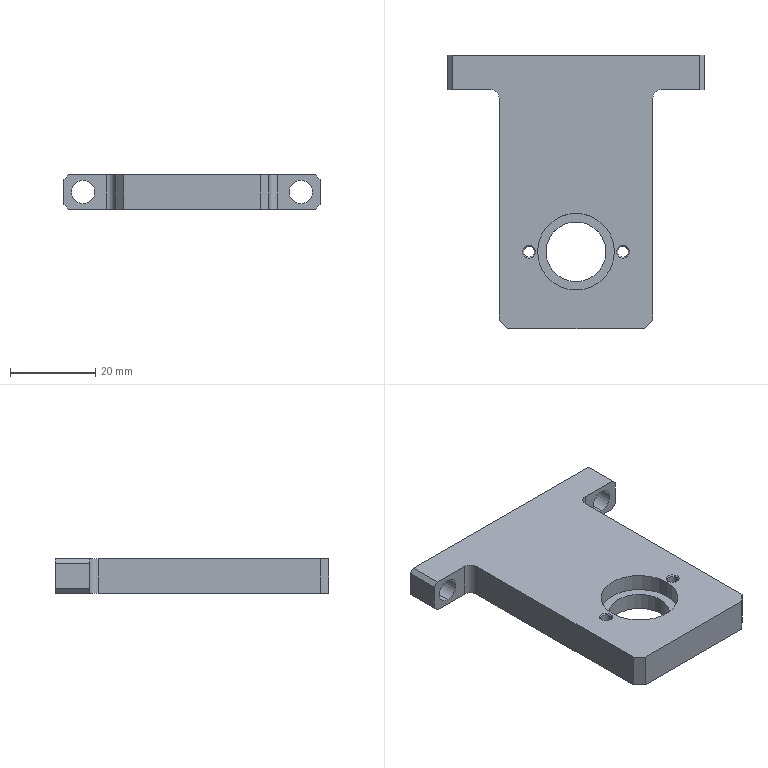Part | STEP file | FBDS-CS-017 | 1 solid | 35 faces | box 60 x 64 x 8 mm | volume 17841 mm3 | plane 17 | cylinder 14 | cone 4 | commonest cylinder face diameters 2.5 x4 5.5 x4 4 x2 14 x2 18 x2
STEP:
#1=CARTESIAN_POINT('',(-12.25,-14.,7.725));
#2=VERTEX_POINT('',#1);
#3=CARTESIAN_POINT('',(-9.75,-14.,7.725));
#4=VERTEX_POINT('',#3);
#5=CARTESIAN_POINT('',(-11.,-14.,7.725));
#6=DIRECTION('',(0.,0.,1.));
#7=DIRECTION('',(1.,0.,0.));
#8=AXIS2_PLACEMENT_3D('',#5,#6,#7);
#9=CIRCLE('',#8,1.25);
#10=EDGE_CURVE('',#2,#4,#9,.T.);
#11=ORIENTED_EDGE('',*,*,#10,.F.);
#12=CARTESIAN_POINT('',(-12.525,-14.,8.));
#13=VERTEX_POINT('',#12);
#14=CARTESIAN_POINT('',(-12.525,-14.,8.));
#15=DIRECTION('',(-0.7071,0.,0.7071));
#16=VECTOR('',#15,1000.);
#17=LINE('',#14,#16);
#18=EDGE_CURVE('',#2,#13,#17,.T.);
#19=ORIENTED_EDGE('',*,*,#18,.T.);
#20=CARTESIAN_POINT('',(-9.475,-14.,8.));
#21=VERTEX_POINT('',#20);
#22=CARTESIAN_POINT('',(-11.,-14.,8.));
#23=DIRECTION('',(0.,0.,1.));
#24=DIRECTION('',(1.,0.,0.));
#25=AXIS2_PLACEMENT_3D('',#22,#23,#24);
#26=CIRCLE('',#25,1.525);
#27=EDGE_CURVE('',#13,#21,#26,.T.);
#28=ORIENTED_EDGE('',*,*,#27,.T.);
#29=CARTESIAN_POINT('',(-9.475,-14.,8.));
#30=DIRECTION('',(0.7071,0.,0.7071));
#31=VECTOR('',#30,1000.);
#32=LINE('',#29,#31);
#33=EDGE_CURVE('',#4,#21,#32,.T.);
#34=ORIENTED_EDGE('',*,*,#33,.F.);
#35=EDGE_LOOP('',(#11,#19,#28,#34));
#36=FACE_OUTER_BOUND('',#35,.T.);
#37=CARTESIAN_POINT('',(-11.,-14.,8.));
#38=DIRECTION('',(0.,0.,1.));
#39=DIRECTION('',(1.,0.,0.));
#40=AXIS2_PLACEMENT_3D('',#37,#38,#39);
#41=CONICAL_SURFACE('',#40,1.525,0.7854);
#42=ADVANCED_FACE('',(#36),#41,.F.);
#43=CARTESIAN_POINT('',(-12.25,-14.,0.));
#44=VERTEX_POINT('',#43);
#45=CARTESIAN_POINT('',(-9.75,-14.,0.));
#46=VERTEX_POINT('',#45);
#47=CARTESIAN_POINT('',(-11.,-14.,0.));
#48=DIRECTION('',(0.,0.,1.));
#49=DIRECTION('',(1.,0.,0.));
#50=AXIS2_PLACEMENT_3D('',#47,#48,#49);
#51=CIRCLE('',#50,1.25);
#52=EDGE_CURVE('',#44,#46,#51,.T.);
#53=ORIENTED_EDGE('',*,*,#52,.F.);
#54=CARTESIAN_POINT('',(-12.25,-14.,8.));
#55=DIRECTION('',(0.,0.,1.));
#56=VECTOR('',#55,1000.);
#57=LINE('',#54,#56);
#58=EDGE_CURVE('',#44,#2,#57,.T.);
#59=ORIENTED_EDGE('',*,*,#58,.T.);
#60=ORIENTED_EDGE('',*,*,#10,.T.);
#61=CARTESIAN_POINT('',(-9.75,-14.,8.));
#62=DIRECTION('',(0.,0.,1.));
#63=VECTOR('',#62,1000.);
#64=LINE('',#61,#63);
#65=EDGE_CURVE('',#46,#4,#64,.T.);
#66=ORIENTED_EDGE('',*,*,#65,.F.);
#67=EDGE_LOOP('',(#53,#59,#60,#66));
#68=FACE_OUTER_BOUND('',#67,.T.);
#69=CARTESIAN_POINT('',(-11.,-14.,8.));
#70=DIRECTION('',(0.,0.,1.));
#71=DIRECTION('',(1.,0.,0.));
#72=AXIS2_PLACEMENT_3D('',#69,#70,#71);
#73=CYLINDRICAL_SURFACE('',#72,1.25);
#74=ADVANCED_FACE('',(#68),#73,.F.);
#75=CARTESIAN_POINT('',(9.75,-14.,7.725));
#76=VERTEX_POINT('',#75);
#77=CARTESIAN_POINT('',(12.25,-14.,7.725));
#78=VERTEX_POINT('',#77);
#79=CARTESIAN_POINT('',(11.,-14.,7.725));
#80=DIRECTION('',(0.,0.,1.));
#81=DIRECTION('',(1.,0.,0.));
#82=AXIS2_PLACEMENT_3D('',#79,#80,#81);
#83=CIRCLE('',#82,1.25);
#84=EDGE_CURVE('',#76,#78,#83,.T.);
#85=ORIENTED_EDGE('',*,*,#84,.F.);
#86=CARTESIAN_POINT('',(9.475,-14.,8.));
#87=VERTEX_POINT('',#86);
#88=CARTESIAN_POINT('',(9.475,-14.,8.));
#89=DIRECTION('',(-0.7071,0.,0.7071));
#90=VECTOR('',#89,1000.);
#91=LINE('',#88,#90);
#92=EDGE_CURVE('',#76,#87,#91,.T.);
#93=ORIENTED_EDGE('',*,*,#92,.T.);
#94=CARTESIAN_POINT('',(12.525,-14.,8.));
#95=VERTEX_POINT('',#94);
#96=CARTESIAN_POINT('',(11.,-14.,8.));
#97=DIRECTION('',(0.,0.,1.));
#98=DIRECTION('',(1.,0.,0.));
#99=AXIS2_PLACEMENT_3D('',#96,#97,#98);
#100=CIRCLE('',#99,1.525);
#101=EDGE_CURVE('',#87,#95,#100,.T.);
#102=ORIENTED_EDGE('',*,*,#101,.T.);
#103=CARTESIAN_POINT('',(12.525,-14.,8.));
#104=DIRECTION('',(0.7071,0.,0.7071));
#105=VECTOR('',#104,1000.);
#106=LINE('',#103,#105);
#107=EDGE_CURVE('',#78,#95,#106,.T.);
#108=ORIENTED_EDGE('',*,*,#107,.F.);
#109=EDGE_LOOP('',(#85,#93,#102,#108));
#110=FACE_OUTER_BOUND('',#109,.T.);
#111=CARTESIAN_POINT('',(11.,-14.,8.));
#112=DIRECTION('',(0.,0.,1.));
#113=DIRECTION('',(1.,0.,0.));
#114=AXIS2_PLACEMENT_3D('',#111,#112,#113);
#115=CONICAL_SURFACE('',#114,1.525,0.7854);
#116=ADVANCED_FACE('',(#110),#115,.F.);
#117=CARTESIAN_POINT('',(9.75,-14.,0.));
#118=VERTEX_POINT('',#117);
#119=CARTESIAN_POINT('',(12.25,-14.,0.));
#120=VERTEX_POINT('',#119);
#121=CARTESIAN_POINT('',(11.,-14.,0.));
#122=DIRECTION('',(0.,0.,1.));
#123=DIRECTION('',(1.,0.,0.));
#124=AXIS2_PLACEMENT_3D('',#121,#122,#123);
#125=CIRCLE('',#124,1.25);
#126=EDGE_CURVE('',#118,#120,#125,.T.);
#127=ORIENTED_EDGE('',*,*,#126,.F.);
#128=CARTESIAN_POINT('',(9.75,-14.,8.));
#129=DIRECTION('',(0.,0.,1.));
#130=VECTOR('',#129,1000.);
#131=LINE('',#128,#130);
#132=EDGE_CURVE('',#118,#76,#131,.T.);
#133=ORIENTED_EDGE('',*,*,#132,.T.);
#134=ORIENTED_EDGE('',*,*,#84,.T.);
#135=CARTESIAN_POINT('',(12.25,-14.,8.));
#136=DIRECTION('',(0.,0.,1.));
#137=VECTOR('',#136,1000.);
#138=LINE('',#135,#137);
#139=EDGE_CURVE('',#120,#78,#138,.T.);
#140=ORIENTED_EDGE('',*,*,#139,.F.);
#141=EDGE_LOOP('',(#127,#133,#134,#140));
#142=FACE_OUTER_BOUND('',#141,.T.);
#143=CARTESIAN_POINT('',(11.,-14.,8.));
#144=DIRECTION('',(0.,0.,1.));
#145=DIRECTION('',(1.,0.,0.));
#146=AXIS2_PLACEMENT_3D('',#143,#144,#145);
#147=CYLINDRICAL_SURFACE('',#146,1.25);
#148=ADVANCED_FACE('',(#142),#147,.F.);
#149=CARTESIAN_POINT('',(-25.5,32.,6.75));
#150=VERTEX_POINT('',#149);
#151=CARTESIAN_POINT('',(-25.5,32.,1.25));
#152=VERTEX_POINT('',#151);
#153=CARTESIAN_POINT('',(-25.5,32.,4.));
#154=DIRECTION('',(0.,-1.,0.));
#155=DIRECTION('',(0.,0.,-1.));
#156=AXIS2_PLACEMENT_3D('',#153,#154,#155);
#157=CIRCLE('',#156,2.75);
#158=EDGE_CURVE('',#150,#152,#157,.T.);
#159=ORIENTED_EDGE('',*,*,#158,.F.);
#160=CARTESIAN_POINT('',(-25.5,24.,6.75));
#161=VERTEX_POINT('',#160);
#162=CARTESIAN_POINT('',(-25.5,24.,6.75));
#163=DIRECTION('',(0.,-1.,0.));
#164=VECTOR('',#163,1000.);
#165=LINE('',#162,#164);
#166=EDGE_CURVE('',#150,#161,#165,.T.);
#167=ORIENTED_EDGE('',*,*,#166,.T.);
#168=CARTESIAN_POINT('',(-25.5,24.,1.25));
#169=VERTEX_POINT('',#168);
#170=CARTESIAN_POINT('',(-25.5,24.,4.));
#171=DIRECTION('',(0.,-1.,0.));
#172=DIRECTION('',(0.,0.,-1.));
#173=AXIS2_PLACEMENT_3D('',#170,#171,#172);
#174=CIRCLE('',#173,2.75);
#175=EDGE_CURVE('',#161,#169,#174,.T.);
#176=ORIENTED_EDGE('',*,*,#175,.T.);
#177=CARTESIAN_POINT('',(-25.5,24.,1.25));
#178=DIRECTION('',(0.,-1.,0.));
#179=VECTOR('',#178,1000.);
#180=LINE('',#177,#179);
#181=EDGE_CURVE('',#152,#169,#180,.T.);
#182=ORIENTED_EDGE('',*,*,#181,.F.);
#183=EDGE_LOOP('',(#159,#167,#176,#182));
#184=FACE_OUTER_BOUND('',#183,.T.);
#185=CARTESIAN_POINT('',(-25.5,24.,4.));
#186=DIRECTION('',(0.,-1.,0.));
#187=DIRECTION('',(0.,0.,-1.));
#188=AXIS2_PLACEMENT_3D('',#185,#186,#187);
#189=CYLINDRICAL_SURFACE('',#188,2.75);
#190=ADVANCED_FACE('',(#184),#189,.F.);
#191=CARTESIAN_POINT('',(25.5,32.,6.75));
#192=VERTEX_POINT('',#191);
#193=CARTESIAN_POINT('',(25.5,32.,1.25));
#194=VERTEX_POINT('',#193);
#195=CARTESIAN_POINT('',(25.5,32.,4.));
#196=DIRECTION('',(0.,-1.,0.));
#197=DIRECTION('',(0.,0.,-1.));
#198=AXIS2_PLACEMENT_3D('',#195,#196,#197);
#199=CIRCLE('',#198,2.75);
#200=EDGE_CURVE('',#192,#194,#199,.T.);
#201=ORIENTED_EDGE('',*,*,#200,.F.);
#202=CARTESIAN_POINT('',(25.5,24.,6.75));
#203=VERTEX_POINT('',#202);
#204=CARTESIAN_POINT('',(25.5,24.,6.75));
#205=DIRECTION('',(0.,-1.,0.));
#206=VECTOR('',#205,1000.);
#207=LINE('',#204,#206);
#208=EDGE_CURVE('',#192,#203,#207,.T.);
#209=ORIENTED_EDGE('',*,*,#208,.T.);
#210=CARTESIAN_POINT('',(25.5,24.,1.25));
#211=VERTEX_POINT('',#210);
#212=CARTESIAN_POINT('',(25.5,24.,4.));
#213=DIRECTION('',(0.,-1.,0.));
#214=DIRECTION('',(0.,0.,-1.));
#215=AXIS2_PLACEMENT_3D('',#212,#213,#214);
#216=CIRCLE('',#215,2.75);
#217=EDGE_CURVE('',#203,#211,#216,.T.);
#218=ORIENTED_EDGE('',*,*,#217,.T.);
#219=CARTESIAN_POINT('',(25.5,24.,1.25));
#220=DIRECTION('',(0.,-1.,0.));
#221=VECTOR('',#220,1000.);
#222=LINE('',#219,#221);
#223=EDGE_CURVE('',#194,#211,#222,.T.);
#224=ORIENTED_EDGE('',*,*,#223,.F.);
#225=EDGE_LOOP('',(#201,#209,#218,#224));
#226=FACE_OUTER_BOUND('',#225,.T.);
#227=CARTESIAN_POINT('',(25.5,24.,4.));
#228=DIRECTION('',(0.,-1.,0.));
#229=DIRECTION('',(0.,0.,-1.));
#230=AXIS2_PLACEMENT_3D('',#227,#228,#229);
#231=CYLINDRICAL_SURFACE('',#230,2.75);
#232=ADVANCED_FACE('',(#226),#231,.F.);
#233=CARTESIAN_POINT('',(7.,-14.,4.));
#234=VERTEX_POINT('',#233);
#235=CARTESIAN_POINT('',(-7.,-14.,4.));
#236=VERTEX_POINT('',#235);
#237=CARTESIAN_POINT('',(0.,-14.,4.));
#238=DIRECTION('',(0.,0.,-1.));
#239=DIRECTION('',(-1.,0.,0.));
#240=AXIS2_PLACEMENT_3D('',#237,#238,#239);
#241=CIRCLE('',#240,7.);
#242=EDGE_CURVE('',#234,#236,#241,.T.);
#243=ORIENTED_EDGE('',*,*,#242,.F.);
#244=CARTESIAN_POINT('',(7.,-14.,0.));
#245=VERTEX_POINT('',#244);
#246=CARTESIAN_POINT('',(7.,-14.,4.));
#247=DIRECTION('',(0.,0.,-1.));
#248=VECTOR('',#247,1000.);
#249=LINE('',#246,#248);
#250=EDGE_CURVE('',#234,#245,#249,.T.);
#251=ORIENTED_EDGE('',*,*,#250,.T.);
#252=CARTESIAN_POINT('',(-7.,-14.,0.));
#253=VERTEX_POINT('',#252);
#254=CARTESIAN_POINT('',(0.,-14.,0.));
#255=DIRECTION('',(0.,0.,-1.));
#256=DIRECTION('',(-1.,0.,0.));
#257=AXIS2_PLACEMENT_3D('',#254,#255,#256);
#258=CIRCLE('',#257,7.);
#259=EDGE_CURVE('',#245,#253,#258,.T.);
#260=ORIENTED_EDGE('',*,*,#259,.T.);
#261=CARTESIAN_POINT('',(-7.,-14.,4.));
#262=DIRECTION('',(0.,0.,-1.));
#263=VECTOR('',#262,1000.);
#264=LINE('',#261,#263);
#265=EDGE_CURVE('',#236,#253,#264,.T.);
#266=ORIENTED_EDGE('',*,*,#265,.F.);
#267=EDGE_LOOP('',(#243,#251,#260,#266));
#268=FACE_OUTER_BOUND('',#267,.T.);
#269=CARTESIAN_POINT('',(0.,-14.,4.));
#270=DIRECTION('',(0.,0.,-1.));
#271=DIRECTION('',(-1.,0.,0.));
#272=AXIS2_PLACEMENT_3D('',#269,#270,#271);
#273=CYLINDRICAL_SURFACE('',#272,7.);
#274=ADVANCED_FACE('',(#268),#273,.F.);
#275=CARTESIAN_POINT('',(-9.,-14.,4.));
#276=VERTEX_POINT('',#275);
#277=CARTESIAN_POINT('',(9.,-14.,4.));
#278=VERTEX_POINT('',#277);
#279=CARTESIAN_POINT('',(0.,-14.,4.));
#280=DIRECTION('',(0.,0.,1.));
#281=DIRECTION('',(-1.,0.,0.));
#282=AXIS2_PLACEMENT_3D('',#279,#280,#281);
#283=CIRCLE('',#282,9.);
#284=EDGE_CURVE('',#276,#278,#283,.T.);
#285=ORIENTED_EDGE('',*,*,#284,.F.);
#286=CARTESIAN_POINT('',(-9.,-14.,8.));
#287=VERTEX_POINT('',#286);
#288=CARTESIAN_POINT('',(-9.,-14.,-2.));
#289=DIRECTION('',(0.,0.,1.));
#290=VECTOR('',#289,1000.);
#291=LINE('',#288,#290);
#292=EDGE_CURVE('',#276,#287,#291,.T.);
#293=ORIENTED_EDGE('',*,*,#292,.T.);
#294=CARTESIAN_POINT('',(9.,-14.,8.));
#295=VERTEX_POINT('',#294);
#296=CARTESIAN_POINT('',(0.,-14.,8.));
#297=DIRECTION('',(0.,0.,1.));
#298=DIRECTION('',(1.,0.,0.));
#299=AXIS2_PLACEMENT_3D('',#296,#297,#298);
#300=CIRCLE('',#299,9.);
#301=EDGE_CURVE('',#287,#295,#300,.T.);
#302=ORIENTED_EDGE('',*,*,#301,.T.);
#303=CARTESIAN_POINT('',(9.,-14.,-2.));
#304=DIRECTION('',(0.,0.,1.));
#305=VECTOR('',#304,1000.);
#306=LINE('',#303,#305);
#307=EDGE_CURVE('',#278,#295,#306,.T.);
#308=ORIENTED_EDGE('',*,*,#307,.F.);
#309=EDGE_LOOP('',(#285,#293,#302,#308));
#310=FACE_OUTER_BOUND('',#309,.T.);
#311=CARTESIAN_POINT('',(0.,-14.,-2.));
#312=DIRECTION('',(0.,0.,1.));
#313=DIRECTION('',(1.,0.,0.));
#314=AXIS2_PLACEMENT_3D('',#311,#312,#313);
#315=CYLINDRICAL_SURFACE('',#314,9.);
#316=ADVANCED_FACE('',(#310),#315,.F.);
#317=ORIENTED_EDGE('',*,*,#292,.F.);
#318=CARTESIAN_POINT('',(0.,-14.,4.));
#319=DIRECTION('',(0.,0.,1.));
#320=DIRECTION('',(-1.,0.,0.));
#321=AXIS2_PLACEMENT_3D('',#318,#319,#320);
#322=CIRCLE('',#321,9.);
#323=EDGE_CURVE('',#278,#276,#322,.T.);
#324=ORIENTED_EDGE('',*,*,#323,.F.);
#325=ORIENTED_EDGE('',*,*,#307,.T.);
#326=CARTESIAN_POINT('',(0.,-14.,8.));
#327=DIRECTION('',(0.,0.,1.));
#328=DIRECTION('',(1.,0.,0.));
#329=AXIS2_PLACEMENT_3D('',#326,#327,#328);
#330=CIRCLE('',#329,9.);
#331=EDGE_CURVE('',#295,#287,#330,.T.);
#332=ORIENTED_EDGE('',*,*,#331,.T.);
#333=EDGE_LOOP('',(#317,#324,#325,#332));
#334=FACE_OUTER_BOUND('',#333,.T.);
#335=CARTESIAN_POINT('',(0.,-14.,-2.));
#336=DIRECTION('',(0.,0.,1.));
#337=DIRECTION('',(1.,0.,0.));
#338=AXIS2_PLACEMENT_3D('',#335,#336,#337);
#339=CYLINDRICAL_SURFACE('',#338,9.);
#340=ADVANCED_FACE('',(#334),#339,.F.);
#341=CARTESIAN_POINT('',(30.,32.,7.));
#342=VERTEX_POINT('',#341);
#343=CARTESIAN_POINT('',(30.,32.,1.));
#344=VERTEX_POINT('',#343);
#345=CARTESIAN_POINT('',(30.,32.,8.));
#346=DIRECTION('',(0.,0.,-1.));
#347=VECTOR('',#346,1000.);
#348=LINE('',#345,#347);
#349=EDGE_CURVE('',#342,#344,#348,.T.);
#350=ORIENTED_EDGE('',*,*,#349,.F.);
#351=CARTESIAN_POINT('',(30.,24.,7.));
#352=VERTEX_POINT('',#351);
#353=CARTESIAN_POINT('',(30.,-32.,7.));
#354=DIRECTION('',(0.,-1.,0.));
#355=VECTOR('',#354,1000.);
#356=LINE('',#353,#355);
#357=EDGE_CURVE('',#342,#352,#356,.T.);
#358=ORIENTED_EDGE('',*,*,#357,.T.);
#359=CARTESIAN_POINT('',(30.,24.,1.));
#360=VERTEX_POINT('',#359);
#361=CARTESIAN_POINT('',(30.,24.,-10.));
#362=DIRECTION('',(0.,0.,1.));
#363=VECTOR('',#362,1000.);
#364=LINE('',#361,#363);
#365=EDGE_CURVE('',#360,#352,#364,.T.);
#366=ORIENTED_EDGE('',*,*,#365,.F.);
#367=CARTESIAN_POINT('',(30.,32.,1.));
#368=DIRECTION('',(0.,1.,0.));
#369=VECTOR('',#368,1000.);
#370=LINE('',#367,#369);
#371=EDGE_CURVE('',#360,#344,#370,.T.);
#372=ORIENTED_EDGE('',*,*,#371,.T.);
#373=EDGE_LOOP('',(#350,#358,#366,#372));
#374=FACE_OUTER_BOUND('',#373,.T.);
#375=CARTESIAN_POINT('',(30.,-32.,8.));
#376=DIRECTION('',(-1.,0.,0.));
#377=DIRECTION('',(0.,0.,1.));
#378=AXIS2_PLACEMENT_3D('',#375,#376,#377);
#379=PLANE('',#378);
#380=ADVANCED_FACE('',(#374),#379,.F.);
#381=CARTESIAN_POINT('',(-25.5,32.,4.));
#382=DIRECTION('',(0.,-1.,0.));
#383=DIRECTION('',(0.,0.,-1.));
#384=AXIS2_PLACEMENT_3D('',#381,#382,#383);
#385=CIRCLE('',#384,2.75);
#386=EDGE_CURVE('',#152,#150,#385,.T.);
#387=ORIENTED_EDGE('',*,*,#386,.T.);
#388=ORIENTED_EDGE('',*,*,#158,.T.);
#389=EDGE_LOOP('',(#387,#388));
#390=FACE_BOUND('',#389,.T.);
#391=CARTESIAN_POINT('',(25.5,32.,4.));
#392=DIRECTION('',(0.,-1.,0.));
#393=DIRECTION('',(0.,0.,-1.));
#394=AXIS2_PLACEMENT_3D('',#391,#392,#393);
#395=CIRCLE('',#394,2.75);
#396=EDGE_CURVE('',#194,#192,#395,.T.);
#397=ORIENTED_EDGE('',*,*,#396,.T.);
#398=ORIENTED_EDGE('',*,*,#200,.T.);
#399=EDGE_LOOP('',(#397,#398));
#400=FACE_BOUND('',#399,.T.);
#401=CARTESIAN_POINT('',(-30.,32.,7.));
#402=VERTEX_POINT('',#401);
#403=CARTESIAN_POINT('',(-30.,32.,1.));
#404=VERTEX_POINT('',#403);
#405=CARTESIAN_POINT('',(-30.,32.,8.));
#406=DIRECTION('',(0.,0.,-1.));
#407=VECTOR('',#406,1000.);
#408=LINE('',#405,#407);
#409=EDGE_CURVE('',#402,#404,#408,.T.);
#410=ORIENTED_EDGE('',*,*,#409,.F.);
#411=CARTESIAN_POINT('',(-29.,32.,8.));
#412=VERTEX_POINT('',#411);
#413=CARTESIAN_POINT('',(-29.,32.,8.));
#414=DIRECTION('',(0.7071,0.,0.7071));
#415=VECTOR('',#414,1000.);
#416=LINE('',#413,#415);
#417=EDGE_CURVE('',#402,#412,#416,.T.);
#418=ORIENTED_EDGE('',*,*,#417,.T.);
#419=CARTESIAN_POINT('',(29.,32.,8.));
#420=VERTEX_POINT('',#419);
#421=CARTESIAN_POINT('',(-30.,32.,8.));
#422=DIRECTION('',(-1.,0.,0.));
#423=VECTOR('',#422,1000.);
#424=LINE('',#421,#423);
#425=EDGE_CURVE('',#420,#412,#424,.T.);
#426=ORIENTED_EDGE('',*,*,#425,.F.);
#427=CARTESIAN_POINT('',(29.,32.,8.));
#428=DIRECTION('',(0.7071,0.,-0.7071));
#429=VECTOR('',#428,1000.);
#430=LINE('',#427,#429);
#431=EDGE_CURVE('',#420,#342,#430,.T.);
#432=ORIENTED_EDGE('',*,*,#431,.T.);
#433=ORIENTED_EDGE('',*,*,#349,.T.);
#434=CARTESIAN_POINT('',(29.,32.,0.));
#435=VERTEX_POINT('',#434);
#436=CARTESIAN_POINT('',(30.,32.,1.));
#437=DIRECTION('',(-0.7071,0.,-0.7071));
#438=VECTOR('',#437,1000.);
#439=LINE('',#436,#438);
#440=EDGE_CURVE('',#344,#435,#439,.T.);
#441=ORIENTED_EDGE('',*,*,#440,.T.);
#442=CARTESIAN_POINT('',(-29.,32.,0.));
#443=VERTEX_POINT('',#442);
#444=CARTESIAN_POINT('',(-30.,32.,0.));
#445=DIRECTION('',(-1.,0.,0.));
#446=VECTOR('',#445,1000.);
#447=LINE('',#444,#446);
#448=EDGE_CURVE('',#435,#443,#447,.T.);
#449=ORIENTED_EDGE('',*,*,#448,.T.);
#450=CARTESIAN_POINT('',(-30.,32.,1.));
#451=DIRECTION('',(-0.7071,0.,0.7071));
#452=VECTOR('',#451,1000.);
#453=LINE('',#450,#452);
#454=EDGE_CURVE('',#443,#404,#453,.T.);
#455=ORIENTED_EDGE('',*,*,#454,.T.);
#456=EDGE_LOOP('',(#410,#418,#426,#432,#433,#441,#449,#455));
#457=FACE_OUTER_BOUND('',#456,.T.);
#458=CARTESIAN_POINT('',(-30.,32.,8.));
#459=DIRECTION('',(0.,-1.,0.));
#460=DIRECTION('',(0.,0.,-1.));
#461=AXIS2_PLACEMENT_3D('',#458,#459,#460);
#462=PLANE('',#461);
#463=ADVANCED_FACE('',(#390,#400,#457),#462,.F.);
#464=CARTESIAN_POINT('',(-30.,24.,1.));
#465=VERTEX_POINT('',#464);
#466=CARTESIAN_POINT('',(-30.,24.,7.));
#467=VERTEX_POINT('',#466);
#468=CARTESIAN_POINT('',(-30.,24.,-10.));
#469=DIRECTION('',(0.,0.,1.));
#470=VECTOR('',#469,1000.);
#471=LINE('',#468,#470);
#472=EDGE_CURVE('',#465,#467,#471,.T.);
#473=ORIENTED_EDGE('',*,*,#472,.T.);
#474=CARTESIAN_POINT('',(-30.,-32.,7.));
#475=DIRECTION('',(0.,1.,0.));
#476=VECTOR('',#475,1000.);
#477=LINE('',#474,#476);
#478=EDGE_CURVE('',#467,#402,#477,.T.);
#479=ORIENTED_EDGE('',*,*,#478,.T.);
#480=ORIENTED_EDGE('',*,*,#409,.T.);
#481=CARTESIAN_POINT('',(-30.,24.,1.));
#482=DIRECTION('',(0.,-1.,0.));
#483=VECTOR('',#482,1000.);
#484=LINE('',#481,#483);
#485=EDGE_CURVE('',#404,#465,#484,.T.);
#486=ORIENTED_EDGE('',*,*,#485,.T.);
#487=EDGE_LOOP('',(#473,#479,#480,#486));
#488=FACE_OUTER_BOUND('',#487,.T.);
#489=CARTESIAN_POINT('',(-30.,-32.,8.));
#490=DIRECTION('',(1.,0.,0.));
#491=DIRECTION('',(0.,0.,-1.));
#492=AXIS2_PLACEMENT_3D('',#489,#490,#491);
#493=PLANE('',#492);
#494=ADVANCED_FACE('',(#488),#493,.F.);
#495=CARTESIAN_POINT('',(-16.,-32.,0.));
#496=VERTEX_POINT('',#495);
#497=CARTESIAN_POINT('',(16.,-32.,0.));
#498=VERTEX_POINT('',#497);
#499=CARTESIAN_POINT('',(-30.,-32.,0.));
#500=DIRECTION('',(1.,0.,0.));
#501=VECTOR('',#500,1000.);
#502=LINE('',#499,#501);
#503=EDGE_CURVE('',#496,#498,#502,.T.);
#504=ORIENTED_EDGE('',*,*,#503,.T.);
#505=CARTESIAN_POINT('',(16.,-32.,8.));
#506=VERTEX_POINT('',#505);
#507=CARTESIAN_POINT('',(16.,-32.,8.));
#508=DIRECTION('',(0.,0.,1.));
#509=VECTOR('',#508,1000.);
#510=LINE('',#507,#509);
#511=EDGE_CURVE('',#498,#506,#510,.T.);
#512=ORIENTED_EDGE('',*,*,#511,.T.);
#513=CARTESIAN_POINT('',(-16.,-32.,8.));
#514=VERTEX_POINT('',#513);
#515=CARTESIAN_POINT('',(-30.,-32.,8.));
#516=DIRECTION('',(1.,0.,0.));
#517=VECTOR('',#516,1000.);
#518=LINE('',#515,#517);
#519=EDGE_CURVE('',#514,#506,#518,.T.);
#520=ORIENTED_EDGE('',*,*,#519,.F.);
#521=CARTESIAN_POINT('',(-16.,-32.,8.));
#522=DIRECTION('',(0.,0.,-1.));
#523=VECTOR('',#522,1000.);
#524=LINE('',#521,#523);
#525=EDGE_CURVE('',#514,#496,#524,.T.);
#526=ORIENTED_EDGE('',*,*,#525,.T.);
#527=EDGE_LOOP('',(#504,#512,#520,#526));
#528=FACE_OUTER_BOUND('',#527,.T.);
#529=CARTESIAN_POINT('',(-30.,-32.,8.));
#530=DIRECTION('',(0.,1.,0.));
#531=DIRECTION('',(0.,0.,1.));
#532=AXIS2_PLACEMENT_3D('',#529,#530,#531);
#533=PLANE('',#532);
#534=ADVANCED_FACE('',(#528),#533,.F.);
#535=CARTESIAN_POINT('',(-11.,-14.,8.));
#536=DIRECTION('',(0.,0.,1.));
#537=DIRECTION('',(1.,0.,0.));
#538=AXIS2_PLACEMENT_3D('',#535,#536,#537);
#539=CIRCLE('',#538,1.525);
#540=EDGE_CURVE('',#21,#13,#539,.T.);
#541=ORIENTED_EDGE('',*,*,#540,.F.);
#542=ORIENTED_EDGE('',*,*,#27,.F.);
#543=EDGE_LOOP('',(#541,#542));
#544=FACE_BOUND('',#543,.T.);
#545=CARTESIAN_POINT('',(11.,-14.,8.));
#546=DIRECTION('',(0.,0.,1.));
#547=DIRECTION('',(1.,0.,0.));
#548=AXIS2_PLACEMENT_3D('',#545,#546,#547);
#549=CIRCLE('',#548,1.525);
#550=EDGE_CURVE('',#95,#87,#549,.T.);
#551=ORIENTED_EDGE('',*,*,#550,.F.);
#552=ORIENTED_EDGE('',*,*,#101,.F.);
#553=EDGE_LOOP('',(#551,#552));
#554=FACE_BOUND('',#553,.T.);
#555=ORIENTED_EDGE('',*,*,#331,.F.);
#556=ORIENTED_EDGE('',*,*,#301,.F.);
#557=EDGE_LOOP('',(#555,#556));
#558=FACE_BOUND('',#557,.T.);
#559=ORIENTED_EDGE('',*,*,#425,.T.);
#560=CARTESIAN_POINT('',(-29.,24.,8.));
#561=VERTEX_POINT('',#560);
#562=CARTESIAN_POINT('',(-29.,0.,8.));
#563=DIRECTION('',(0.,-1.,0.));
#564=VECTOR('',#563,1000.);
#565=LINE('',#562,#564);
#566=EDGE_CURVE('',#412,#561,#565,.T.);
#567=ORIENTED_EDGE('',*,*,#566,.T.);
#568=CARTESIAN_POINT('',(-20.,24.,8.));
#569=VERTEX_POINT('',#568);
#570=CARTESIAN_POINT('',(-30.,24.,8.));
#571=DIRECTION('',(-1.,0.,0.));
#572=VECTOR('',#571,1000.);
#573=LINE('',#570,#572);
#574=EDGE_CURVE('',#569,#561,#573,.T.);
#575=ORIENTED_EDGE('',*,*,#574,.F.);
#576=CARTESIAN_POINT('',(-18.,22.,8.));
#577=VERTEX_POINT('',#576);
#578=CARTESIAN_POINT('',(-20.,22.,8.));
#579=DIRECTION('',(0.,0.,-1.));
#580=DIRECTION('',(-1.,0.,0.));
#581=AXIS2_PLACEMENT_3D('',#578,#579,#580);
#582=CIRCLE('',#581,2.);
#583=EDGE_CURVE('',#569,#577,#582,.T.);
#584=ORIENTED_EDGE('',*,*,#583,.T.);
#585=CARTESIAN_POINT('',(-18.,-30.,8.));
#586=VERTEX_POINT('',#585);
#587=CARTESIAN_POINT('',(-18.,-32.,8.));
#588=DIRECTION('',(0.,1.,0.));
#589=VECTOR('',#588,1000.);
#590=LINE('',#587,#589);
#591=EDGE_CURVE('',#586,#577,#590,.T.);
#592=ORIENTED_EDGE('',*,*,#591,.F.);
#593=CARTESIAN_POINT('',(-18.,-30.,8.));
#594=DIRECTION('',(0.7071,-0.7071,0.));
#595=VECTOR('',#594,1000.);
#596=LINE('',#593,#595);
#597=EDGE_CURVE('',#586,#514,#596,.T.);
#598=ORIENTED_EDGE('',*,*,#597,.T.);
#599=ORIENTED_EDGE('',*,*,#519,.T.);
#600=CARTESIAN_POINT('',(18.,-30.,8.));
#601=VERTEX_POINT('',#600);
#602=CARTESIAN_POINT('',(16.,-32.,8.));
#603=DIRECTION('',(0.7071,0.7071,0.));
#604=VECTOR('',#603,1000.);
#605=LINE('',#602,#604);
#606=EDGE_CURVE('',#506,#601,#605,.T.);
#607=ORIENTED_EDGE('',*,*,#606,.T.);
#608=CARTESIAN_POINT('',(18.,22.,8.));
#609=VERTEX_POINT('',#608);
#610=CARTESIAN_POINT('',(18.,-32.,8.));
#611=DIRECTION('',(0.,-1.,0.));
#612=VECTOR('',#611,1000.);
#613=LINE('',#610,#612);
#614=EDGE_CURVE('',#609,#601,#613,.T.);
#615=ORIENTED_EDGE('',*,*,#614,.F.);
#616=CARTESIAN_POINT('',(20.,24.,8.));
#617=VERTEX_POINT('',#616);
#618=CARTESIAN_POINT('',(20.,22.,8.));
#619=DIRECTION('',(0.,0.,-1.));
#620=DIRECTION('',(-1.,0.,0.));
#621=AXIS2_PLACEMENT_3D('',#618,#619,#620);
#622=CIRCLE('',#621,2.);
#623=EDGE_CURVE('',#609,#617,#622,.T.);
#624=ORIENTED_EDGE('',*,*,#623,.T.);
#625=CARTESIAN_POINT('',(29.,24.,8.));
#626=VERTEX_POINT('',#625);
#627=CARTESIAN_POINT('',(30.,24.,8.));
#628=DIRECTION('',(-1.,0.,0.));
#629=VECTOR('',#628,1000.);
#630=LINE('',#627,#629);
#631=EDGE_CURVE('',#626,#617,#630,.T.);
#632=ORIENTED_EDGE('',*,*,#631,.F.);
#633=CARTESIAN_POINT('',(29.,0.,8.));
#634=DIRECTION('',(0.,1.,0.));
#635=VECTOR('',#634,1000.);
#636=LINE('',#633,#635);
#637=EDGE_CURVE('',#626,#420,#636,.T.);
#638=ORIENTED_EDGE('',*,*,#637,.T.);
#639=EDGE_LOOP('',(#559,#567,#575,#584,#592,#598,#599,#607,#615,#624,#632,#638));
#640=FACE_OUTER_BOUND('',#639,.T.);
#641=CARTESIAN_POINT('',(0.,0.,8.));
#642=DIRECTION('',(0.,0.,-1.));
#643=DIRECTION('',(-1.,0.,0.));
#644=AXIS2_PLACEMENT_3D('',#641,#642,#643);
#645=PLANE('',#644);
#646=ADVANCED_FACE('',(#544,#554,#558,#640),#645,.F.);
#647=CARTESIAN_POINT('',(-11.,-14.,0.));
#648=DIRECTION('',(0.,0.,1.));
#649=DIRECTION('',(1.,0.,0.));
#650=AXIS2_PLACEMENT_3D('',#647,#648,#649);
#651=CIRCLE('',#650,1.25);
#652=EDGE_CURVE('',#46,#44,#651,.T.);
#653=ORIENTED_EDGE('',*,*,#652,.T.);
#654=ORIENTED_EDGE('',*,*,#52,.T.);
#655=EDGE_LOOP('',(#653,#654));
#656=FACE_BOUND('',#655,.T.);
#657=CARTESIAN_POINT('',(11.,-14.,0.));
#658=DIRECTION('',(0.,0.,1.));
#659=DIRECTION('',(1.,0.,0.));
#660=AXIS2_PLACEMENT_3D('',#657,#658,#659);
#661=CIRCLE('',#660,1.25);
#662=EDGE_CURVE('',#120,#118,#661,.T.);
#663=ORIENTED_EDGE('',*,*,#662,.T.);
#664=ORIENTED_EDGE('',*,*,#126,.T.);
#665=EDGE_LOOP('',(#663,#664));
#666=FACE_BOUND('',#665,.T.);
#667=CARTESIAN_POINT('',(-29.,24.,0.));
#668=VERTEX_POINT('',#667);
#669=CARTESIAN_POINT('',(-20.,24.,0.));
#670=VERTEX_POINT('',#669);
#671=CARTESIAN_POINT('',(0.,24.,0.));
#672=DIRECTION('',(1.,0.,0.));
#673=VECTOR('',#672,1000.);
#674=LINE('',#671,#673);
#675=EDGE_CURVE('',#668,#670,#674,.T.);
#676=ORIENTED_EDGE('',*,*,#675,.F.);
#677=CARTESIAN_POINT('',(-29.,32.,0.));
#678=DIRECTION('',(0.,1.,0.));
#679=VECTOR('',#678,1000.);
#680=LINE('',#677,#679);
#681=EDGE_CURVE('',#668,#443,#680,.T.);
#682=ORIENTED_EDGE('',*,*,#681,.T.);
#683=ORIENTED_EDGE('',*,*,#448,.F.);
#684=CARTESIAN_POINT('',(29.,24.,0.));
#685=VERTEX_POINT('',#684);
#686=CARTESIAN_POINT('',(29.,24.,0.));
#687=DIRECTION('',(0.,-1.,0.));
#688=VECTOR('',#687,1000.);
#689=LINE('',#686,#688);
#690=EDGE_CURVE('',#435,#685,#689,.T.);
#691=ORIENTED_EDGE('',*,*,#690,.T.);
#692=CARTESIAN_POINT('',(20.,24.,0.));
#693=VERTEX_POINT('',#692);
#694=CARTESIAN_POINT('',(0.,24.,0.));
#695=DIRECTION('',(1.,0.,0.));
#696=VECTOR('',#695,1000.);
#697=LINE('',#694,#696);
#698=EDGE_CURVE('',#693,#685,#697,.T.);
#699=ORIENTED_EDGE('',*,*,#698,.F.);
#700=CARTESIAN_POINT('',(18.,22.,0.));
#701=VERTEX_POINT('',#700);
#702=CARTESIAN_POINT('',(20.,22.,0.));
#703=DIRECTION('',(0.,0.,1.));
#704=DIRECTION('',(-1.,0.,0.));
#705=AXIS2_PLACEMENT_3D('',#702,#703,#704);
#706=CIRCLE('',#705,2.);
#707=EDGE_CURVE('',#693,#701,#706,.T.);
#708=ORIENTED_EDGE('',*,*,#707,.T.);
#709=CARTESIAN_POINT('',(18.,-30.,0.));
#710=VERTEX_POINT('',#709);
#711=CARTESIAN_POINT('',(18.,0.,0.));
#712=DIRECTION('',(0.,1.,0.));
#713=VECTOR('',#712,1000.);
#714=LINE('',#711,#713);
#715=EDGE_CURVE('',#710,#701,#714,.T.);
#716=ORIENTED_EDGE('',*,*,#715,.F.);
#717=CARTESIAN_POINT('',(24.,-24.,0.));
#718=DIRECTION('',(-0.7071,-0.7071,0.));
#719=VECTOR('',#718,1000.);
#720=LINE('',#717,#719);
#721=EDGE_CURVE('',#710,#498,#720,.T.);
#722=ORIENTED_EDGE('',*,*,#721,.T.);
#723=ORIENTED_EDGE('',*,*,#503,.F.);
#724=CARTESIAN_POINT('',(-18.,-30.,0.));
#725=VERTEX_POINT('',#724);
#726=CARTESIAN_POINT('',(-24.,-24.,0.));
#727=DIRECTION('',(-0.7071,0.7071,0.));
#728=VECTOR('',#727,1000.);
#729=LINE('',#726,#728);
#730=EDGE_CURVE('',#496,#725,#729,.T.);
#731=ORIENTED_EDGE('',*,*,#730,.T.);
#732=CARTESIAN_POINT('',(-18.,22.,0.));
#733=VERTEX_POINT('',#732);
#734=CARTESIAN_POINT('',(-18.,0.,0.));
#735=DIRECTION('',(0.,-1.,0.));
#736=VECTOR('',#735,1000.);
#737=LINE('',#734,#736);
#738=EDGE_CURVE('',#733,#725,#737,.T.);
#739=ORIENTED_EDGE('',*,*,#738,.F.);
#740=CARTESIAN_POINT('',(-20.,22.,0.));
#741=DIRECTION('',(0.,0.,1.));
#742=DIRECTION('',(-1.,0.,0.));
#743=AXIS2_PLACEMENT_3D('',#740,#741,#742);
#744=CIRCLE('',#743,2.);
#745=EDGE_CURVE('',#733,#670,#744,.T.);
#746=ORIENTED_EDGE('',*,*,#745,.T.);
#747=EDGE_LOOP('',(#676,#682,#683,#691,#699,#708,#716,#722,#723,#731,#739,#746));
#748=FACE_OUTER_BOUND('',#747,.T.);
#749=CARTESIAN_POINT('',(0.,-14.,0.));
#750=DIRECTION('',(0.,0.,-1.));
#751=DIRECTION('',(-1.,0.,0.));
#752=AXIS2_PLACEMENT_3D('',#749,#750,#751);
#753=CIRCLE('',#752,7.);
#754=EDGE_CURVE('',#253,#245,#753,.T.);
#755=ORIENTED_EDGE('',*,*,#754,.F.);
#756=ORIENTED_EDGE('',*,*,#259,.F.);
#757=EDGE_LOOP('',(#755,#756));
#758=FACE_BOUND('',#757,.T.);
#759=CARTESIAN_POINT('',(0.,0.,0.));
#760=DIRECTION('',(0.,0.,-1.));
#761=DIRECTION('',(-1.,0.,0.));
#762=AXIS2_PLACEMENT_3D('',#759,#760,#761);
#763=PLANE('',#762);
#764=ADVANCED_FACE('',(#656,#666,#748,#758),#763,.T.);
#765=ORIENTED_EDGE('',*,*,#715,.T.);
#766=CARTESIAN_POINT('',(18.,22.,8.));
#767=DIRECTION('',(0.,0.,1.));
#768=VECTOR('',#767,1000.);
#769=LINE('',#766,#768);
#770=EDGE_CURVE('',#701,#609,#769,.T.);
#771=ORIENTED_EDGE('',*,*,#770,.T.);
#772=ORIENTED_EDGE('',*,*,#614,.T.);
#773=CARTESIAN_POINT('',(18.,-30.,-10.));
#774=DIRECTION('',(0.,0.,-1.));
#775=VECTOR('',#774,1000.);
#776=LINE('',#773,#775);
#777=EDGE_CURVE('',#601,#710,#776,.T.);
#778=ORIENTED_EDGE('',*,*,#777,.T.);
#779=EDGE_LOOP('',(#765,#771,#772,#778));
#780=FACE_OUTER_BOUND('',#779,.T.);
#781=CARTESIAN_POINT('',(18.,-32.,-10.));
#782=DIRECTION('',(-1.,0.,0.));
#783=DIRECTION('',(0.,0.,1.));
#784=AXIS2_PLACEMENT_3D('',#781,#782,#783);
#785=PLANE('',#784);
#786=ADVANCED_FACE('',(#780),#785,.F.);
#787=CARTESIAN_POINT('',(25.5,24.,4.));
#788=DIRECTION('',(0.,-1.,0.));
#789=DIRECTION('',(0.,0.,-1.));
#790=AXIS2_PLACEMENT_3D('',#787,#788,#789);
#791=CIRCLE('',#790,2.75);
#792=EDGE_CURVE('',#211,#203,#791,.T.);
#793=ORIENTED_EDGE('',*,*,#792,.F.);
#794=ORIENTED_EDGE('',*,*,#217,.F.);
#795=EDGE_LOOP('',(#793,#794));
#796=FACE_BOUND('',#795,.T.);
#797=ORIENTED_EDGE('',*,*,#631,.T.);
#798=CARTESIAN_POINT('',(20.,24.,0.));
#799=DIRECTION('',(0.,0.,-1.));
#800=VECTOR('',#799,1000.);
#801=LINE('',#798,#800);
#802=EDGE_CURVE('',#617,#693,#801,.T.);
#803=ORIENTED_EDGE('',*,*,#802,.T.);
#804=ORIENTED_EDGE('',*,*,#698,.T.);
#805=CARTESIAN_POINT('',(30.,24.,1.));
#806=DIRECTION('',(0.7071,0.,0.7071));
#807=VECTOR('',#806,1000.);
#808=LINE('',#805,#807);
#809=EDGE_CURVE('',#685,#360,#808,.T.);
#810=ORIENTED_EDGE('',*,*,#809,.T.);
#811=ORIENTED_EDGE('',*,*,#365,.T.);
#812=CARTESIAN_POINT('',(29.,24.,8.));
#813=DIRECTION('',(-0.7071,0.,0.7071));
#814=VECTOR('',#813,1000.);
#815=LINE('',#812,#814);
#816=EDGE_CURVE('',#352,#626,#815,.T.);
#817=ORIENTED_EDGE('',*,*,#816,.T.);
#818=EDGE_LOOP('',(#797,#803,#804,#810,#811,#817));
#819=FACE_OUTER_BOUND('',#818,.T.);
#820=CARTESIAN_POINT('',(30.,24.,-10.));
#821=DIRECTION('',(0.,1.,0.));
#822=DIRECTION('',(0.,0.,1.));
#823=AXIS2_PLACEMENT_3D('',#820,#821,#822);
#824=PLANE('',#823);
#825=ADVANCED_FACE('',(#796,#819),#824,.F.);
#826=CARTESIAN_POINT('',(-25.5,24.,4.));
#827=DIRECTION('',(0.,-1.,0.));
#828=DIRECTION('',(0.,0.,-1.));
#829=AXIS2_PLACEMENT_3D('',#826,#827,#828);
#830=CIRCLE('',#829,2.75);
#831=EDGE_CURVE('',#169,#161,#830,.T.);
#832=ORIENTED_EDGE('',*,*,#831,.F.);
#833=ORIENTED_EDGE('',*,*,#175,.F.);
#834=EDGE_LOOP('',(#832,#833));
#835=FACE_BOUND('',#834,.T.);
#836=ORIENTED_EDGE('',*,*,#675,.T.);
#837=CARTESIAN_POINT('',(-20.,24.,8.));
#838=DIRECTION('',(0.,0.,1.));
#839=VECTOR('',#838,1000.);
#840=LINE('',#837,#839);
#841=EDGE_CURVE('',#670,#569,#840,.T.);
#842=ORIENTED_EDGE('',*,*,#841,.T.);
#843=ORIENTED_EDGE('',*,*,#574,.T.);
#844=CARTESIAN_POINT('',(-29.,24.,8.));
#845=DIRECTION('',(-0.7071,0.,-0.7071));
#846=VECTOR('',#845,1000.);
#847=LINE('',#844,#846);
#848=EDGE_CURVE('',#561,#467,#847,.T.);
#849=ORIENTED_EDGE('',*,*,#848,.T.);
#850=ORIENTED_EDGE('',*,*,#472,.F.);
#851=CARTESIAN_POINT('',(-30.,24.,1.));
#852=DIRECTION('',(0.7071,0.,-0.7071));
#853=VECTOR('',#852,1000.);
#854=LINE('',#851,#853);
#855=EDGE_CURVE('',#465,#668,#854,.T.);
#856=ORIENTED_EDGE('',*,*,#855,.T.);
#857=EDGE_LOOP('',(#836,#842,#843,#849,#850,#856));
#858=FACE_OUTER_BOUND('',#857,.T.);
#859=CARTESIAN_POINT('',(-30.,24.,-10.));
#860=DIRECTION('',(0.,1.,0.));
#861=DIRECTION('',(0.,0.,1.));
#862=AXIS2_PLACEMENT_3D('',#859,#860,#861);
#863=PLANE('',#862);
#864=ADVANCED_FACE('',(#835,#858),#863,.F.);
#865=ORIENTED_EDGE('',*,*,#591,.T.);
#866=CARTESIAN_POINT('',(-18.,22.,0.));
#867=DIRECTION('',(0.,0.,-1.));
#868=VECTOR('',#867,1000.);
#869=LINE('',#866,#868);
#870=EDGE_CURVE('',#577,#733,#869,.T.);
#871=ORIENTED_EDGE('',*,*,#870,.T.);
#872=ORIENTED_EDGE('',*,*,#738,.T.);
#873=CARTESIAN_POINT('',(-18.,-30.,-10.));
#874=DIRECTION('',(0.,0.,1.));
#875=VECTOR('',#874,1000.);
#876=LINE('',#873,#875);
#877=EDGE_CURVE('',#725,#586,#876,.T.);
#878=ORIENTED_EDGE('',*,*,#877,.T.);
#879=EDGE_LOOP('',(#865,#871,#872,#878));
#880=FACE_OUTER_BOUND('',#879,.T.);
#881=CARTESIAN_POINT('',(-18.,-32.,-10.));
#882=DIRECTION('',(1.,0.,0.));
#883=DIRECTION('',(0.,0.,-1.));
#884=AXIS2_PLACEMENT_3D('',#881,#882,#883);
#885=PLANE('',#884);
#886=ADVANCED_FACE('',(#880),#885,.F.);
#887=CARTESIAN_POINT('',(0.,-14.,4.));
#888=DIRECTION('',(0.,0.,-1.));
#889=DIRECTION('',(-1.,0.,0.));
#890=AXIS2_PLACEMENT_3D('',#887,#888,#889);
#891=CIRCLE('',#890,7.);
#892=EDGE_CURVE('',#236,#234,#891,.T.);
#893=ORIENTED_EDGE('',*,*,#892,.T.);
#894=ORIENTED_EDGE('',*,*,#242,.T.);
#895=EDGE_LOOP('',(#893,#894));
#896=FACE_BOUND('',#895,.T.);
#897=ORIENTED_EDGE('',*,*,#323,.T.);
#898=ORIENTED_EDGE('',*,*,#284,.T.);
#899=EDGE_LOOP('',(#897,#898));
#900=FACE_OUTER_BOUND('',#899,.T.);
#901=CARTESIAN_POINT('',(0.,-14.,4.));
#902=DIRECTION('',(0.,0.,-1.));
#903=DIRECTION('',(-1.,0.,0.));
#904=AXIS2_PLACEMENT_3D('',#901,#902,#903);
#905=PLANE('',#904);
#906=ADVANCED_FACE('',(#896,#900),#905,.F.);
#907=ORIENTED_EDGE('',*,*,#250,.F.);
#908=ORIENTED_EDGE('',*,*,#892,.F.);
#909=ORIENTED_EDGE('',*,*,#265,.T.);
#910=ORIENTED_EDGE('',*,*,#754,.T.);
#911=EDGE_LOOP('',(#907,#908,#909,#910));
#912=FACE_OUTER_BOUND('',#911,.T.);
#913=CARTESIAN_POINT('',(0.,-14.,4.));
#914=DIRECTION('',(0.,0.,-1.));
#915=DIRECTION('',(-1.,0.,0.));
#916=AXIS2_PLACEMENT_3D('',#913,#914,#915);
#917=CYLINDRICAL_SURFACE('',#916,7.);
#918=ADVANCED_FACE('',(#912),#917,.F.);
#919=ORIENTED_EDGE('',*,*,#208,.F.);
#920=ORIENTED_EDGE('',*,*,#396,.F.);
#921=ORIENTED_EDGE('',*,*,#223,.T.);
#922=ORIENTED_EDGE('',*,*,#792,.T.);
#923=EDGE_LOOP('',(#919,#920,#921,#922));
#924=FACE_OUTER_BOUND('',#923,.T.);
#925=CARTESIAN_POINT('',(25.5,24.,4.));
#926=DIRECTION('',(0.,-1.,0.));
#927=DIRECTION('',(0.,0.,-1.));
#928=AXIS2_PLACEMENT_3D('',#925,#926,#927);
#929=CYLINDRICAL_SURFACE('',#928,2.75);
#930=ADVANCED_FACE('',(#924),#929,.F.);
#931=ORIENTED_EDGE('',*,*,#166,.F.);
#932=ORIENTED_EDGE('',*,*,#386,.F.);
#933=ORIENTED_EDGE('',*,*,#181,.T.);
#934=ORIENTED_EDGE('',*,*,#831,.T.);
#935=EDGE_LOOP('',(#931,#932,#933,#934));
#936=FACE_OUTER_BOUND('',#935,.T.);
#937=CARTESIAN_POINT('',(-25.5,24.,4.));
#938=DIRECTION('',(0.,-1.,0.));
#939=DIRECTION('',(0.,0.,-1.));
#940=AXIS2_PLACEMENT_3D('',#937,#938,#939);
#941=CYLINDRICAL_SURFACE('',#940,2.75);
#942=ADVANCED_FACE('',(#936),#941,.F.);
#943=ORIENTED_EDGE('',*,*,#721,.F.);
#944=ORIENTED_EDGE('',*,*,#777,.F.);
#945=ORIENTED_EDGE('',*,*,#606,.F.);
#946=ORIENTED_EDGE('',*,*,#511,.F.);
#947=EDGE_LOOP('',(#943,#944,#945,#946));
#948=FACE_OUTER_BOUND('',#947,.T.);
#949=CARTESIAN_POINT('',(16.,-32.,8.));
#950=DIRECTION('',(-0.7071,0.7071,0.));
#951=DIRECTION('',(0.,0.,1.));
#952=AXIS2_PLACEMENT_3D('',#949,#950,#951);
#953=PLANE('',#952);
#954=ADVANCED_FACE('',(#948),#953,.F.);
#955=ORIENTED_EDGE('',*,*,#730,.F.);
#956=ORIENTED_EDGE('',*,*,#525,.F.);
#957=ORIENTED_EDGE('',*,*,#597,.F.);
#958=ORIENTED_EDGE('',*,*,#877,.F.);
#959=EDGE_LOOP('',(#955,#956,#957,#958));
#960=FACE_OUTER_BOUND('',#959,.T.);
#961=CARTESIAN_POINT('',(-18.,-30.,-10.));
#962=DIRECTION('',(0.7071,0.7071,0.));
#963=DIRECTION('',(0.,0.,1.));
#964=AXIS2_PLACEMENT_3D('',#961,#962,#963);
#965=PLANE('',#964);
#966=ADVANCED_FACE('',(#960),#965,.F.);
#967=ORIENTED_EDGE('',*,*,#417,.F.);
#968=ORIENTED_EDGE('',*,*,#478,.F.);
#969=ORIENTED_EDGE('',*,*,#848,.F.);
#970=ORIENTED_EDGE('',*,*,#566,.F.);
#971=EDGE_LOOP('',(#967,#968,#969,#970));
#972=FACE_OUTER_BOUND('',#971,.T.);
#973=CARTESIAN_POINT('',(-29.,0.,8.));
#974=DIRECTION('',(0.7071,0.,-0.7071));
#975=DIRECTION('',(0.,-1.,0.));
#976=AXIS2_PLACEMENT_3D('',#973,#974,#975);
#977=PLANE('',#976);
#978=ADVANCED_FACE('',(#972),#977,.F.);
#979=ORIENTED_EDGE('',*,*,#454,.F.);
#980=ORIENTED_EDGE('',*,*,#681,.F.);
#981=ORIENTED_EDGE('',*,*,#855,.F.);
#982=ORIENTED_EDGE('',*,*,#485,.F.);
#983=EDGE_LOOP('',(#979,#980,#981,#982));
#984=FACE_OUTER_BOUND('',#983,.T.);
#985=CARTESIAN_POINT('',(-30.,-32.,1.));
#986=DIRECTION('',(-0.7071,0.,-0.7071));
#987=DIRECTION('',(0.,1.,0.));
#988=AXIS2_PLACEMENT_3D('',#985,#986,#987);
#989=PLANE('',#988);
#990=ADVANCED_FACE('',(#984),#989,.T.);
#991=ORIENTED_EDGE('',*,*,#816,.F.);
#992=ORIENTED_EDGE('',*,*,#357,.F.);
#993=ORIENTED_EDGE('',*,*,#431,.F.);
#994=ORIENTED_EDGE('',*,*,#637,.F.);
#995=EDGE_LOOP('',(#991,#992,#993,#994));
#996=FACE_OUTER_BOUND('',#995,.T.);
#997=CARTESIAN_POINT('',(29.,0.,8.));
#998=DIRECTION('',(-0.7071,0.,-0.7071));
#999=DIRECTION('',(0.,1.,0.));
#1000=AXIS2_PLACEMENT_3D('',#997,#998,#999);
#1001=PLANE('',#1000);
#1002=ADVANCED_FACE('',(#996),#1001,.F.);
#1003=ORIENTED_EDGE('',*,*,#809,.F.);
#1004=ORIENTED_EDGE('',*,*,#690,.F.);
#1005=ORIENTED_EDGE('',*,*,#440,.F.);
#1006=ORIENTED_EDGE('',*,*,#371,.F.);
#1007=EDGE_LOOP('',(#1003,#1004,#1005,#1006));
#1008=FACE_OUTER_BOUND('',#1007,.T.);
#1009=CARTESIAN_POINT('',(30.,-32.,1.));
#1010=DIRECTION('',(0.7071,0.,-0.7071));
#1011=DIRECTION('',(0.,-1.,0.));
#1012=AXIS2_PLACEMENT_3D('',#1009,#1010,#1011);
#1013=PLANE('',#1012);
#1014=ADVANCED_FACE('',(#1008),#1013,.T.);
#1015=ORIENTED_EDGE('',*,*,#707,.F.);
#1016=ORIENTED_EDGE('',*,*,#802,.F.);
#1017=ORIENTED_EDGE('',*,*,#623,.F.);
#1018=ORIENTED_EDGE('',*,*,#770,.F.);
#1019=EDGE_LOOP('',(#1015,#1016,#1017,#1018));
#1020=FACE_OUTER_BOUND('',#1019,.T.);
#1021=CARTESIAN_POINT('',(20.,22.,-10.));
#1022=DIRECTION('',(0.,0.,-1.));
#1023=DIRECTION('',(-1.,0.,0.));
#1024=AXIS2_PLACEMENT_3D('',#1021,#1022,#1023);
#1025=CYLINDRICAL_SURFACE('',#1024,2.);
#1026=ADVANCED_FACE('',(#1020),#1025,.F.);
#1027=ORIENTED_EDGE('',*,*,#745,.F.);
#1028=ORIENTED_EDGE('',*,*,#870,.F.);
#1029=ORIENTED_EDGE('',*,*,#583,.F.);
#1030=ORIENTED_EDGE('',*,*,#841,.F.);
#1031=EDGE_LOOP('',(#1027,#1028,#1029,#1030));
#1032=FACE_OUTER_BOUND('',#1031,.T.);
#1033=CARTESIAN_POINT('',(-20.,22.,-10.));
#1034=DIRECTION('',(0.,0.,-1.));
#1035=DIRECTION('',(-1.,0.,0.));
#1036=AXIS2_PLACEMENT_3D('',#1033,#1034,#1035);
#1037=CYLINDRICAL_SURFACE('',#1036,2.);
#1038=ADVANCED_FACE('',(#1032),#1037,.F.);
#1039=ORIENTED_EDGE('',*,*,#132,.F.);
#1040=ORIENTED_EDGE('',*,*,#662,.F.);
#1041=ORIENTED_EDGE('',*,*,#139,.T.);
#1042=CARTESIAN_POINT('',(11.,-14.,7.725));
#1043=DIRECTION('',(0.,0.,1.));
#1044=DIRECTION('',(1.,0.,0.));
#1045=AXIS2_PLACEMENT_3D('',#1042,#1043,#1044);
#1046=CIRCLE('',#1045,1.25);
#1047=EDGE_CURVE('',#78,#76,#1046,.T.);
#1048=ORIENTED_EDGE('',*,*,#1047,.T.);
#1049=EDGE_LOOP('',(#1039,#1040,#1041,#1048));
#1050=FACE_OUTER_BOUND('',#1049,.T.);
#1051=CARTESIAN_POINT('',(11.,-14.,8.));
#1052=DIRECTION('',(0.,0.,1.));
#1053=DIRECTION('',(1.,0.,0.));
#1054=AXIS2_PLACEMENT_3D('',#1051,#1052,#1053);
#1055=CYLINDRICAL_SURFACE('',#1054,1.25);
#1056=ADVANCED_FACE('',(#1050),#1055,.F.);
#1057=ORIENTED_EDGE('',*,*,#92,.F.);
#1058=ORIENTED_EDGE('',*,*,#1047,.F.);
#1059=ORIENTED_EDGE('',*,*,#107,.T.);
#1060=ORIENTED_EDGE('',*,*,#550,.T.);
#1061=EDGE_LOOP('',(#1057,#1058,#1059,#1060));
#1062=FACE_OUTER_BOUND('',#1061,.T.);
#1063=CARTESIAN_POINT('',(11.,-14.,8.));
#1064=DIRECTION('',(0.,0.,1.));
#1065=DIRECTION('',(1.,0.,0.));
#1066=AXIS2_PLACEMENT_3D('',#1063,#1064,#1065);
#1067=CONICAL_SURFACE('',#1066,1.525,0.7854);
#1068=ADVANCED_FACE('',(#1062),#1067,.F.);
#1069=ORIENTED_EDGE('',*,*,#58,.F.);
#1070=ORIENTED_EDGE('',*,*,#652,.F.);
#1071=ORIENTED_EDGE('',*,*,#65,.T.);
#1072=CARTESIAN_POINT('',(-11.,-14.,7.725));
#1073=DIRECTION('',(0.,0.,1.));
#1074=DIRECTION('',(1.,0.,0.));
#1075=AXIS2_PLACEMENT_3D('',#1072,#1073,#1074);
#1076=CIRCLE('',#1075,1.25);
#1077=EDGE_CURVE('',#4,#2,#1076,.T.);
#1078=ORIENTED_EDGE('',*,*,#1077,.T.);
#1079=EDGE_LOOP('',(#1069,#1070,#1071,#1078));
#1080=FACE_OUTER_BOUND('',#1079,.T.);
#1081=CARTESIAN_POINT('',(-11.,-14.,8.));
#1082=DIRECTION('',(0.,0.,1.));
#1083=DIRECTION('',(1.,0.,0.));
#1084=AXIS2_PLACEMENT_3D('',#1081,#1082,#1083);
#1085=CYLINDRICAL_SURFACE('',#1084,1.25);
#1086=ADVANCED_FACE('',(#1080),#1085,.F.);
#1087=ORIENTED_EDGE('',*,*,#18,.F.);
#1088=ORIENTED_EDGE('',*,*,#1077,.F.);
#1089=ORIENTED_EDGE('',*,*,#33,.T.);
#1090=ORIENTED_EDGE('',*,*,#540,.T.);
#1091=EDGE_LOOP('',(#1087,#1088,#1089,#1090));
#1092=FACE_OUTER_BOUND('',#1091,.T.);
#1093=CARTESIAN_POINT('',(-11.,-14.,8.));
#1094=DIRECTION('',(0.,0.,1.));
#1095=DIRECTION('',(1.,0.,0.));
#1096=AXIS2_PLACEMENT_3D('',#1093,#1094,#1095);
#1097=CONICAL_SURFACE('',#1096,1.525,0.7854);
#1098=ADVANCED_FACE('',(#1092),#1097,.F.);
#1099=CLOSED_SHELL('',(#42,#74,#116,#148,#190,#232,#274,#316,#340,#380,#463,#494,#534,#646,#764,#786,#825,#864,#886,#906,#918,#930,#942,#954,#966,#978,#990,#1002,#1014,#1026,#1038,#1056,#1068,#1086,#1098));
#1100=MANIFOLD_SOLID_BREP('',#1099);
#1101=CARTESIAN_POINT('',(0.,0.,0.));
#1102=DIRECTION('',(0.,0.,1.));
#1103=DIRECTION('',(1.,0.,0.));
#1104=AXIS2_PLACEMENT_3D('',#1101,#1102,#1103);
#1105=(LENGTH_UNIT()NAMED_UNIT(*)SI_UNIT(.MILLI.,.METRE.));
#1106=UNCERTAINTY_MEASURE_WITH_UNIT(LENGTH_MEASURE(0.00001),#1105,'','');
#1107=(NAMED_UNIT(*)PLANE_ANGLE_UNIT()SI_UNIT($,.RADIAN.));
#1108=(NAMED_UNIT(*)SI_UNIT($,.STERADIAN.)SOLID_ANGLE_UNIT());
#1109=(GEOMETRIC_REPRESENTATION_CONTEXT(3)GLOBAL_UNCERTAINTY_ASSIGNED_CONTEXT((#1106))GLOBAL_UNIT_ASSIGNED_CONTEXT((#1105,#1107,#1108))REPRESENTATION_CONTEXT('',''));
#1110=ADVANCED_BREP_SHAPE_REPRESENTATION('',(#1100,#1104),#1109);